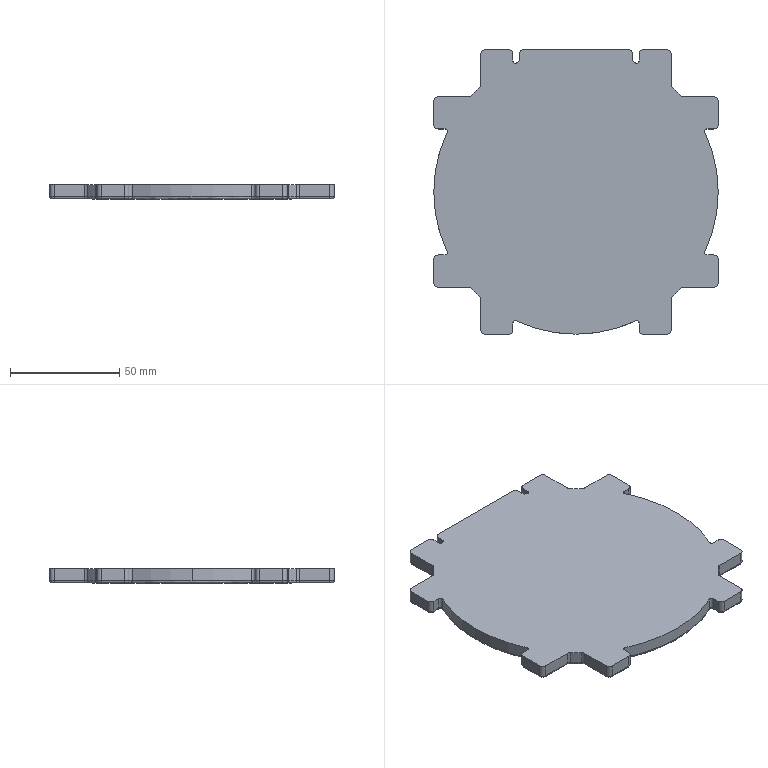Part | STEP file | 31090370--ISMH3-850002 | 1 solid | 155 faces | box 130 x 130 x 6.7 mm | volume 96579 mm3 | cylinder 77 | spline 48 | plane 30 | commonest cylinder face diameters 2 x39 4 x26 130 x10 91.2 x2